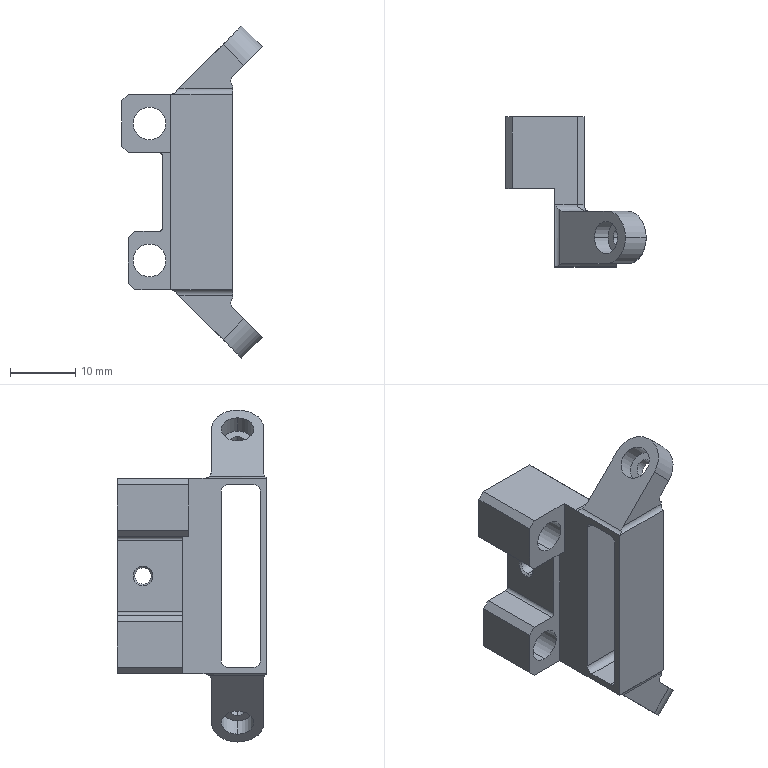Part | 1 solid | 72 faces | box 21.534 x 23 x 50.912 mm | volume 4563 mm3 | cylinder 33 | plane 33 | cone 4 | spline 2 | commonest cylinder face diameters 2 x13 5 x6 2.7 x4 8 x4 1 x2 2.5 x2